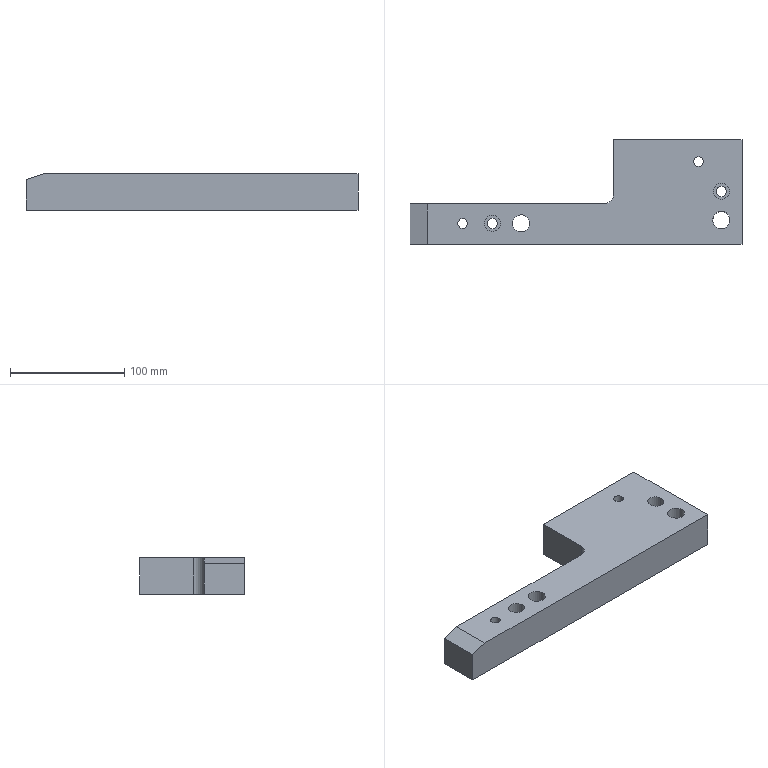Part | STEP file | gslz 2016.10.28-13_id406_x_t | 1 solid | 24 faces | box 290 x 91 x 32 mm | volume 496412 mm3 | plane 13 | cylinder 11 | commonest cylinder face diameters 8.5 x2 9 x2 14 x2 15 x2 20 x2 18 x1